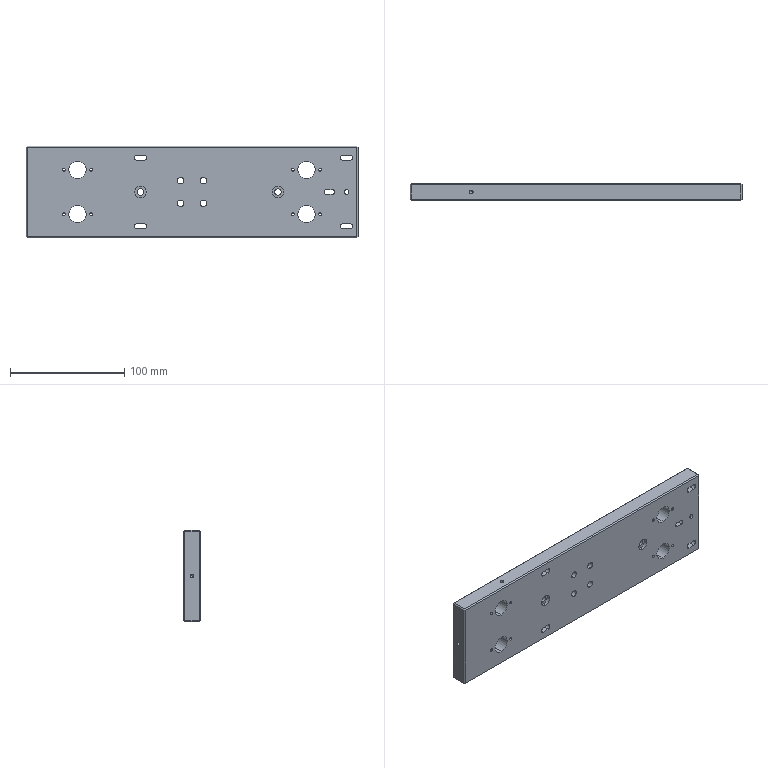Part | STEP file | 01-05 small base plate | 1 solid | 120 faces | box 290 x 15 x 80 mm | volume 328016 mm3 | cylinder 70 | plane 44 | cone 6 | commonest cylinder face diameters 2.5 x16 10 x16 5.8 x12 4.5 x8 15 x8 3.3 x6